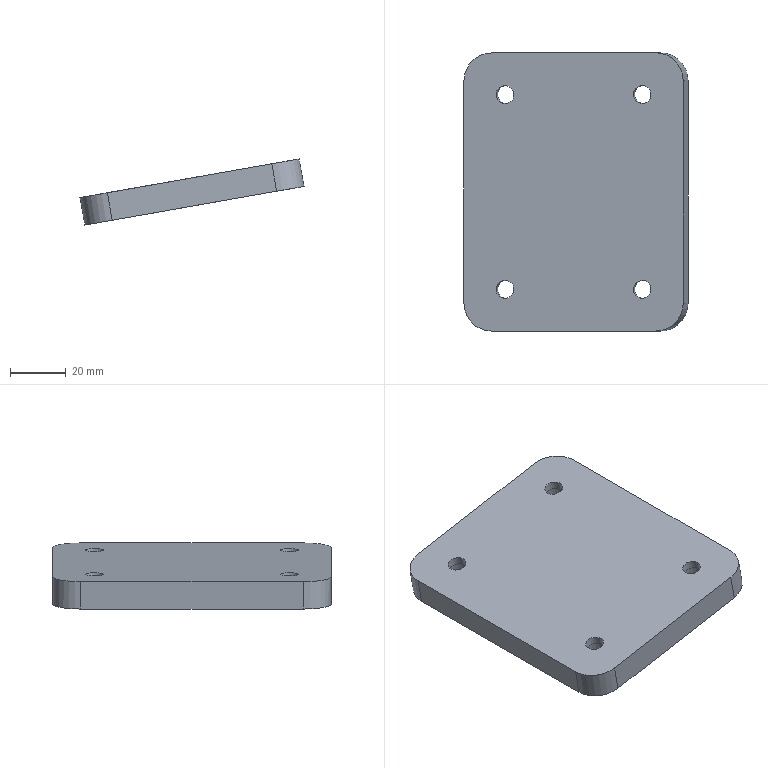Part | STEP file | solid 182 | 1 solid | 22 faces | box 80.521 x 100 x 23.74 mm | volume 76082 mm3 | cylinder 12 | plane 9 | spline 1 | commonest cylinder face diameters 6.5 x4 11 x4 20 x4